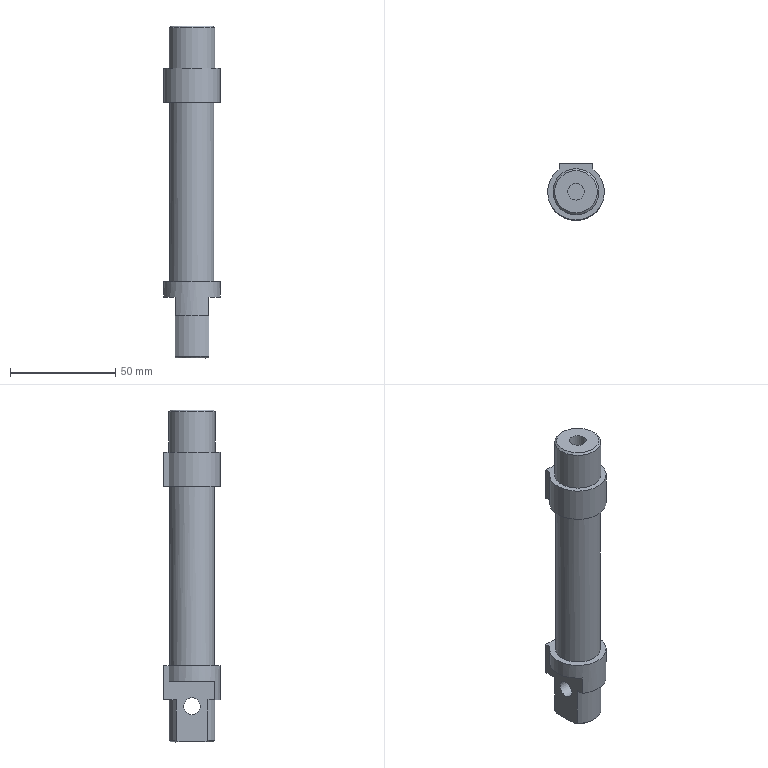Part | STEP file | 1 solid | 35 faces | box 27 x 27 x 158 mm | volume 40169 mm3 | plane 19 | cylinder 11 | cone 5 | commonest cylinder face diameters 22 x3 8 x2 8.566 x2 27 x2 20 x1 21.3 x1